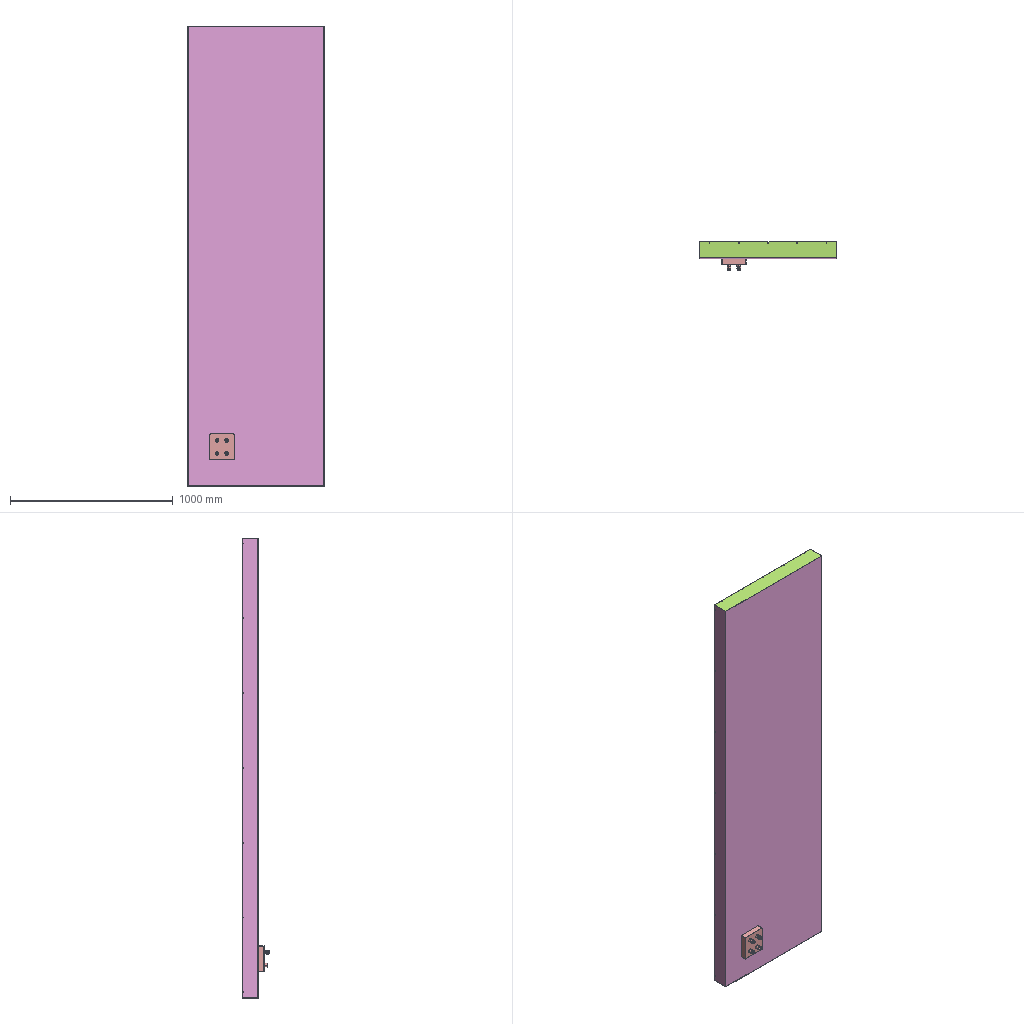Assembly | SolidWorks | 6 different items | 9 placed | box 840 x 172 x 2830 mm
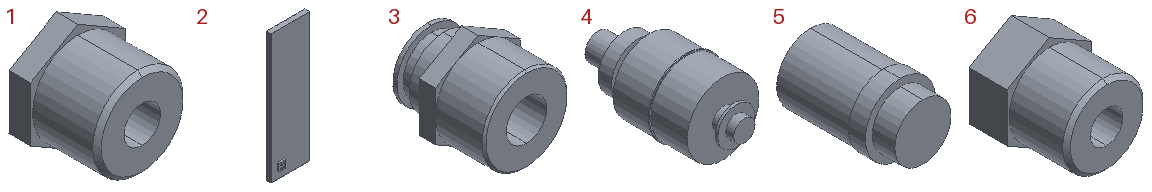Parts list (item | quantity | size | volume | features):
1 | x1 | 22 x 20 x 25.403 mm | 6124 mm3 | features 3DProfileFeature 1, Chamfer 1, Extrusion 1, HoleWzd 1, ICE 1
2 | x1 | 840 x 159 x 2830 mm | 3143571 mm3 | features ICE 6, 3DProfileFeature 3, HoleWzd 3, LPattern 2, Fillet 1, FlatPattern 1, SMBaseFlange 1, SheetMetal 1
3 | x2 | 21 x 24.5 x 24.249 mm | 5082 mm3 | features ICE 6, Chamfer 1, Extrusion 1
4 | x2 | 28 x 55 x 28 mm | 19112 mm3 | features Revolution 1
5 | x2 | 25 x 40 x 25 mm | 17221 mm3 | features Revolution 1
6 | x1 | 22 x 25 x 25.403 mm | 7936 mm3 | features 3DProfileFeature 1, Chamfer 1, Extrusion 1, HoleWzd 1, ICE 1
Mates (type | each side: item.copy, entity, surface, feature):
Concentric | 2.1 face cylinder G1/2 Tapped Hole2 | 6.1 face cylinder Cut-Extrude1
Concentric | 2.1 face cylinder G1/2 Tapped Hole2 | 1.1 face cylinder Cut-Extrude1
Coincident | 2.1 face plane Boss-Extrude12 | 6.1 face plane Cut-Extrude1
Coincident | 2.1 face plane Boss-Extrude12 | 1.1 face plane Cut-Extrude1
Coincident | 1.1 face plane Boss-Extrude1 | 6.1 face plane Boss-Extrude1
Parallel | 2.1 face plane Boss-Extrude9 | 6.1 face plane Boss-Extrude1
Concentric | 6.1 face cylinder M10 Tapped Hole1 | 4.1 face cylinder Revolve1
Coincident | 6.1 face plane Boss-Extrude1 | 4.1 face plane Revolve1
Coincident | 1.1 face plane Boss-Extrude1 | 4.2 face plane Revolve1
Concentric | 1.1 face cylinder M10 Tapped Hole1 | 4.2 face cylinder Revolve1
Concentric | 2.1 face cylinder G1/2 Tapped Hole2 | 5.1 face cylinder Revolve1
Coincident | 2.1 face plane Boss-Extrude12 | 5.1 face plane Revolve1
Concentric | 2.1 face cylinder G1/2 Tapped Hole2 | 5.2 face cylinder Revolve1
Coincident | 5.1 face plane Revolve1 | 5.2 face plane Revolve1
Coincident | 3.1 face plane Boss-Extrude1 | 3.2 face plane Boss-Extrude1
Coincident | 2.1 face plane Boss-Extrude12 | 3.2 face plane Boss-Extrude2
Concentric | 2.1 face cylinder Boss-Extrude12 | 3.1 face cylinder Boss-Extrude1
Concentric | 2.1 face cylinder Boss-Extrude12 | 3.2 face cylinder Boss-Extrude1